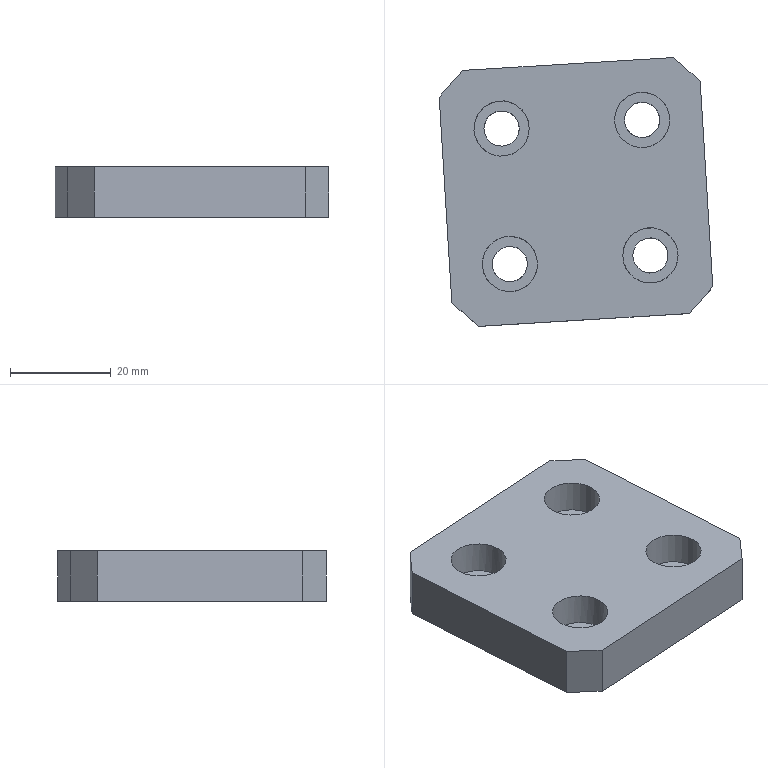Part | STEP file | 车灯-后视镜_id74_x_t | 1 solid | 22 faces | box 54.406 x 53.469 x 10 mm | volume 23010 mm3 | plane 14 | cylinder 8 | commonest cylinder face diameters 7 x4 11 x4
STEP:
#1=CARTESIAN_POINT('',(106.46,-55.923,-255.5));
#2=VERTEX_POINT('',#1);
#3=CARTESIAN_POINT('',(108.963,-96.847,-255.5));
#4=VERTEX_POINT('',#3);
#5=CARTESIAN_POINT('',(107.624,-74.965,-255.5));
#6=DIRECTION('',(0.06105,-0.9981,0.));
#7=VECTOR('',#6,1.);
#8=LINE('',#5,#7);
#9=EDGE_CURVE('',#2,#4,#8,.T.);
#10=ORIENTED_EDGE('',*,*,#9,.F.);
#11=CARTESIAN_POINT('',(101.164,-51.238,-255.5));
#12=VERTEX_POINT('',#11);
#13=CARTESIAN_POINT('',(94.843,-45.646,-255.5));
#14=DIRECTION('',(-0.749,0.6626,0.));
#15=VECTOR('',#14,1.);
#16=LINE('',#13,#15);
#17=EDGE_CURVE('',#2,#12,#16,.T.);
#18=ORIENTED_EDGE('',*,*,#17,.T.);
#19=CARTESIAN_POINT('',(59.242,-53.802,-255.5));
#20=VERTEX_POINT('',#19);
#21=CARTESIAN_POINT('',(65.219,-53.436,-255.5));
#22=DIRECTION('',(0.9981,0.06105,0.));
#23=VECTOR('',#22,1.);
#24=LINE('',#21,#23);
#25=EDGE_CURVE('',#20,#12,#24,.T.);
#26=ORIENTED_EDGE('',*,*,#25,.F.);
#27=CARTESIAN_POINT('',(54.557,-59.098,-255.5));
#28=VERTEX_POINT('',#27);
#29=CARTESIAN_POINT('',(50.767,-63.382,-255.5));
#30=DIRECTION('',(-0.6626,-0.749,0.));
#31=VECTOR('',#30,1.);
#32=LINE('',#29,#31);
#33=EDGE_CURVE('',#20,#28,#32,.T.);
#34=ORIENTED_EDGE('',*,*,#33,.T.);
#35=CARTESIAN_POINT('',(57.06,-100.021,-255.5));
#36=VERTEX_POINT('',#35);
#37=CARTESIAN_POINT('',(55.721,-78.139,-255.5));
#38=DIRECTION('',(-0.06105,0.9981,0.));
#39=VECTOR('',#38,1.);
#40=LINE('',#37,#39);
#41=EDGE_CURVE('',#36,#28,#40,.T.);
#42=ORIENTED_EDGE('',*,*,#41,.F.);
#43=CARTESIAN_POINT('',(62.355,-104.707,-255.5));
#44=VERTEX_POINT('',#43);
#45=CARTESIAN_POINT('',(51.269,-94.898,-255.5));
#46=DIRECTION('',(0.749,-0.6626,0.));
#47=VECTOR('',#46,1.);
#48=LINE('',#45,#47);
#49=EDGE_CURVE('',#36,#44,#48,.T.);
#50=ORIENTED_EDGE('',*,*,#49,.T.);
#51=CARTESIAN_POINT('',(104.277,-102.143,-255.5));
#52=VERTEX_POINT('',#51);
#53=CARTESIAN_POINT('',(68.333,-104.341,-255.5));
#54=DIRECTION('',(-0.9981,-0.06105,0.));
#55=VECTOR('',#54,1.);
#56=LINE('',#53,#55);
#57=EDGE_CURVE('',#52,#44,#56,.T.);
#58=ORIENTED_EDGE('',*,*,#57,.F.);
#59=CARTESIAN_POINT('',(100.019,-106.956,-255.5));
#60=DIRECTION('',(0.6626,0.749,0.));
#61=VECTOR('',#60,1.);
#62=LINE('',#59,#61);
#63=EDGE_CURVE('',#52,#4,#62,.T.);
#64=ORIENTED_EDGE('',*,*,#63,.T.);
#65=EDGE_LOOP('',(#10,#18,#26,#34,#42,#50,#58,#64));
#66=FACE_BOUND('',#65,.T.);
#67=CARTESIAN_POINT('',(74.11,-92.302,-255.5));
#68=VERTEX_POINT('',#67);
#69=CARTESIAN_POINT('',(68.61,-92.302,-255.5));
#70=DIRECTION('',(0.,0.,1.));
#71=DIRECTION('',(1.,0.,0.));
#72=AXIS2_PLACEMENT_3D('',#69,#70,#71);
#73=CIRCLE('',#72,5.5);
#74=EDGE_CURVE('',#68,#68,#73,.T.);
#75=ORIENTED_EDGE('',*,*,#74,.F.);
#76=EDGE_LOOP('',(#75));
#77=FACE_BOUND('',#76,.T.);
#78=CARTESIAN_POINT('',(102.058,-90.592,-255.5));
#79=VERTEX_POINT('',#78);
#80=CARTESIAN_POINT('',(96.558,-90.592,-255.5));
#81=DIRECTION('',(0.,0.,-1.));
#82=DIRECTION('',(1.,0.,0.));
#83=AXIS2_PLACEMENT_3D('',#80,#81,#82);
#84=CIRCLE('',#83,5.5);
#85=EDGE_CURVE('',#79,#79,#84,.T.);
#86=ORIENTED_EDGE('',*,*,#85,.T.);
#87=EDGE_LOOP('',(#86));
#88=FACE_BOUND('',#87,.T.);
#89=CARTESIAN_POINT('',(72.462,-65.352,-255.5));
#90=VERTEX_POINT('',#89);
#91=CARTESIAN_POINT('',(66.962,-65.352,-255.5));
#92=DIRECTION('',(0.,0.,-1.));
#93=DIRECTION('',(1.,0.,0.));
#94=AXIS2_PLACEMENT_3D('',#91,#92,#93);
#95=CIRCLE('',#94,5.5);
#96=EDGE_CURVE('',#90,#90,#95,.T.);
#97=ORIENTED_EDGE('',*,*,#96,.T.);
#98=EDGE_LOOP('',(#97));
#99=FACE_BOUND('',#98,.T.);
#100=CARTESIAN_POINT('',(100.409,-63.643,-255.5));
#101=VERTEX_POINT('',#100);
#102=CARTESIAN_POINT('',(94.909,-63.643,-255.5));
#103=DIRECTION('',(0.,0.,1.));
#104=DIRECTION('',(1.,0.,0.));
#105=AXIS2_PLACEMENT_3D('',#102,#103,#104);
#106=CIRCLE('',#105,5.5);
#107=EDGE_CURVE('',#101,#101,#106,.T.);
#108=ORIENTED_EDGE('',*,*,#107,.F.);
#109=EDGE_LOOP('',(#108));
#110=FACE_BOUND('',#109,.T.);
#111=CARTESIAN_POINT('',(66.689,-77.469,-255.5));
#112=DIRECTION('',(0.,0.,1.));
#113=DIRECTION('',(0.9981,0.06105,0.));
#114=AXIS2_PLACEMENT_3D('',#111,#112,#113);
#115=PLANE('',#114);
#116=ADVANCED_FACE('',(#66,#77,#88,#99,#110),#115,.T.);
#117=CARTESIAN_POINT('',(62.355,-104.707,-265.5));
#118=VERTEX_POINT('',#117);
#119=CARTESIAN_POINT('',(104.277,-102.143,-265.5));
#120=VERTEX_POINT('',#119);
#121=CARTESIAN_POINT('',(68.333,-104.341,-265.5));
#122=DIRECTION('',(0.9981,0.06105,0.));
#123=VECTOR('',#122,1.);
#124=LINE('',#121,#123);
#125=EDGE_CURVE('',#118,#120,#124,.T.);
#126=ORIENTED_EDGE('',*,*,#125,.T.);
#127=CARTESIAN_POINT('',(104.277,-102.143,-267.5));
#128=DIRECTION('',(0.,0.,1.));
#129=VECTOR('',#128,1.);
#130=LINE('',#127,#129);
#131=EDGE_CURVE('',#120,#52,#130,.T.);
#132=ORIENTED_EDGE('',*,*,#131,.T.);
#133=ORIENTED_EDGE('',*,*,#57,.T.);
#134=CARTESIAN_POINT('',(62.355,-104.707,-267.5));
#135=DIRECTION('',(0.,0.,-1.));
#136=VECTOR('',#135,1.);
#137=LINE('',#134,#136);
#138=EDGE_CURVE('',#44,#118,#137,.T.);
#139=ORIENTED_EDGE('',*,*,#138,.T.);
#140=EDGE_LOOP('',(#126,#132,#133,#139));
#141=FACE_OUTER_BOUND('',#140,.T.);
#142=CARTESIAN_POINT('',(68.333,-104.341,-267.5));
#143=DIRECTION('',(0.06105,-0.9981,0.));
#144=DIRECTION('',(0.,0.,-1.));
#145=AXIS2_PLACEMENT_3D('',#142,#143,#144);
#146=PLANE('',#145);
#147=ADVANCED_FACE('',(#141),#146,.T.);
#148=ORIENTED_EDGE('',*,*,#25,.T.);
#149=CARTESIAN_POINT('',(101.164,-51.238,-265.5));
#150=VERTEX_POINT('',#149);
#151=CARTESIAN_POINT('',(101.164,-51.238,-267.5));
#152=DIRECTION('',(0.,0.,-1.));
#153=VECTOR('',#152,1.);
#154=LINE('',#151,#153);
#155=EDGE_CURVE('',#12,#150,#154,.T.);
#156=ORIENTED_EDGE('',*,*,#155,.T.);
#157=CARTESIAN_POINT('',(59.242,-53.802,-265.5));
#158=VERTEX_POINT('',#157);
#159=CARTESIAN_POINT('',(65.219,-53.436,-265.5));
#160=DIRECTION('',(-0.9981,-0.06105,0.));
#161=VECTOR('',#160,1.);
#162=LINE('',#159,#161);
#163=EDGE_CURVE('',#150,#158,#162,.T.);
#164=ORIENTED_EDGE('',*,*,#163,.T.);
#165=CARTESIAN_POINT('',(59.242,-53.802,-267.5));
#166=DIRECTION('',(0.,0.,1.));
#167=VECTOR('',#166,1.);
#168=LINE('',#165,#167);
#169=EDGE_CURVE('',#158,#20,#168,.T.);
#170=ORIENTED_EDGE('',*,*,#169,.T.);
#171=EDGE_LOOP('',(#148,#156,#164,#170));
#172=FACE_OUTER_BOUND('',#171,.T.);
#173=CARTESIAN_POINT('',(65.219,-53.436,-267.5));
#174=DIRECTION('',(-0.06105,0.9981,0.));
#175=DIRECTION('',(0.,0.,1.));
#176=AXIS2_PLACEMENT_3D('',#173,#174,#175);
#177=PLANE('',#176);
#178=ADVANCED_FACE('',(#172),#177,.T.);
#179=ORIENTED_EDGE('',*,*,#163,.F.);
#180=CARTESIAN_POINT('',(106.46,-55.923,-265.5));
#181=VERTEX_POINT('',#180);
#182=CARTESIAN_POINT('',(94.843,-45.646,-265.5));
#183=DIRECTION('',(0.749,-0.6626,0.));
#184=VECTOR('',#183,1.);
#185=LINE('',#182,#184);
#186=EDGE_CURVE('',#150,#181,#185,.T.);
#187=ORIENTED_EDGE('',*,*,#186,.T.);
#188=CARTESIAN_POINT('',(108.963,-96.847,-265.5));
#189=VERTEX_POINT('',#188);
#190=CARTESIAN_POINT('',(107.624,-74.965,-265.5));
#191=DIRECTION('',(-0.06105,0.9981,0.));
#192=VECTOR('',#191,1.);
#193=LINE('',#190,#192);
#194=EDGE_CURVE('',#189,#181,#193,.T.);
#195=ORIENTED_EDGE('',*,*,#194,.F.);
#196=CARTESIAN_POINT('',(100.019,-106.956,-265.5));
#197=DIRECTION('',(-0.6626,-0.749,0.));
#198=VECTOR('',#197,1.);
#199=LINE('',#196,#198);
#200=EDGE_CURVE('',#189,#120,#199,.T.);
#201=ORIENTED_EDGE('',*,*,#200,.T.);
#202=ORIENTED_EDGE('',*,*,#125,.F.);
#203=CARTESIAN_POINT('',(57.06,-100.021,-265.5));
#204=VERTEX_POINT('',#203);
#205=CARTESIAN_POINT('',(51.269,-94.898,-265.5));
#206=DIRECTION('',(-0.749,0.6626,0.));
#207=VECTOR('',#206,1.);
#208=LINE('',#205,#207);
#209=EDGE_CURVE('',#118,#204,#208,.T.);
#210=ORIENTED_EDGE('',*,*,#209,.T.);
#211=CARTESIAN_POINT('',(54.557,-59.098,-265.5));
#212=VERTEX_POINT('',#211);
#213=CARTESIAN_POINT('',(55.721,-78.139,-265.5));
#214=DIRECTION('',(0.06105,-0.9981,0.));
#215=VECTOR('',#214,1.);
#216=LINE('',#213,#215);
#217=EDGE_CURVE('',#212,#204,#216,.T.);
#218=ORIENTED_EDGE('',*,*,#217,.F.);
#219=CARTESIAN_POINT('',(50.767,-63.382,-265.5));
#220=DIRECTION('',(0.6626,0.749,0.));
#221=VECTOR('',#220,1.);
#222=LINE('',#219,#221);
#223=EDGE_CURVE('',#212,#158,#222,.T.);
#224=ORIENTED_EDGE('',*,*,#223,.T.);
#225=EDGE_LOOP('',(#179,#187,#195,#201,#202,#210,#218,#224));
#226=FACE_BOUND('',#225,.T.);
#227=CARTESIAN_POINT('',(65.11,-92.302,-265.5));
#228=VERTEX_POINT('',#227);
#229=CARTESIAN_POINT('',(68.61,-92.302,-265.5));
#230=DIRECTION('',(0.,0.,-1.));
#231=DIRECTION('',(-1.,0.,0.));
#232=AXIS2_PLACEMENT_3D('',#229,#230,#231);
#233=CIRCLE('',#232,3.5);
#234=EDGE_CURVE('',#228,#228,#233,.T.);
#235=ORIENTED_EDGE('',*,*,#234,.F.);
#236=EDGE_LOOP('',(#235));
#237=FACE_BOUND('',#236,.T.);
#238=CARTESIAN_POINT('',(93.058,-90.592,-265.5));
#239=VERTEX_POINT('',#238);
#240=CARTESIAN_POINT('',(96.558,-90.592,-265.5));
#241=DIRECTION('',(0.,0.,1.));
#242=DIRECTION('',(-1.,0.,0.));
#243=AXIS2_PLACEMENT_3D('',#240,#241,#242);
#244=CIRCLE('',#243,3.5);
#245=EDGE_CURVE('',#239,#239,#244,.T.);
#246=ORIENTED_EDGE('',*,*,#245,.T.);
#247=EDGE_LOOP('',(#246));
#248=FACE_BOUND('',#247,.T.);
#249=CARTESIAN_POINT('',(63.462,-65.352,-265.5));
#250=VERTEX_POINT('',#249);
#251=CARTESIAN_POINT('',(66.962,-65.352,-265.5));
#252=DIRECTION('',(0.,0.,1.));
#253=DIRECTION('',(-1.,0.,0.));
#254=AXIS2_PLACEMENT_3D('',#251,#252,#253);
#255=CIRCLE('',#254,3.5);
#256=EDGE_CURVE('',#250,#250,#255,.T.);
#257=ORIENTED_EDGE('',*,*,#256,.T.);
#258=EDGE_LOOP('',(#257));
#259=FACE_BOUND('',#258,.T.);
#260=CARTESIAN_POINT('',(91.409,-63.643,-265.5));
#261=VERTEX_POINT('',#260);
#262=CARTESIAN_POINT('',(94.909,-63.643,-265.5));
#263=DIRECTION('',(0.,0.,-1.));
#264=DIRECTION('',(-1.,0.,0.));
#265=AXIS2_PLACEMENT_3D('',#262,#263,#264);
#266=CIRCLE('',#265,3.5);
#267=EDGE_CURVE('',#261,#261,#266,.T.);
#268=ORIENTED_EDGE('',*,*,#267,.F.);
#269=EDGE_LOOP('',(#268));
#270=FACE_BOUND('',#269,.T.);
#271=CARTESIAN_POINT('',(66.689,-77.469,-265.5));
#272=DIRECTION('',(0.,0.,-1.));
#273=DIRECTION('',(-0.9981,-0.06105,0.));
#274=AXIS2_PLACEMENT_3D('',#271,#272,#273);
#275=PLANE('',#274);
#276=ADVANCED_FACE('',(#226,#237,#248,#259,#270),#275,.T.);
#277=ORIENTED_EDGE('',*,*,#194,.T.);
#278=CARTESIAN_POINT('',(106.46,-55.923,-267.5));
#279=DIRECTION('',(0.,0.,1.));
#280=VECTOR('',#279,1.);
#281=LINE('',#278,#280);
#282=EDGE_CURVE('',#181,#2,#281,.T.);
#283=ORIENTED_EDGE('',*,*,#282,.T.);
#284=ORIENTED_EDGE('',*,*,#9,.T.);
#285=CARTESIAN_POINT('',(108.963,-96.847,-267.5));
#286=DIRECTION('',(0.,0.,-1.));
#287=VECTOR('',#286,1.);
#288=LINE('',#285,#287);
#289=EDGE_CURVE('',#4,#189,#288,.T.);
#290=ORIENTED_EDGE('',*,*,#289,.T.);
#291=EDGE_LOOP('',(#277,#283,#284,#290));
#292=FACE_OUTER_BOUND('',#291,.T.);
#293=CARTESIAN_POINT('',(107.624,-74.965,-267.5));
#294=DIRECTION('',(0.9981,0.06105,0.));
#295=DIRECTION('',(0.,0.,-1.));
#296=AXIS2_PLACEMENT_3D('',#293,#294,#295);
#297=PLANE('',#296);
#298=ADVANCED_FACE('',(#292),#297,.T.);
#299=CARTESIAN_POINT('',(91.416,-63.857,-262.));
#300=VERTEX_POINT('',#299);
#301=CARTESIAN_POINT('',(94.909,-63.643,-262.));
#302=DIRECTION('',(0.,0.,-1.));
#303=DIRECTION('',(-0.9981,-0.06105,0.));
#304=AXIS2_PLACEMENT_3D('',#301,#302,#303);
#305=CIRCLE('',#304,3.5);
#306=EDGE_CURVE('',#300,#300,#305,.T.);
#307=ORIENTED_EDGE('',*,*,#306,.F.);
#308=EDGE_LOOP('',(#307));
#309=FACE_BOUND('',#308,.T.);
#310=ORIENTED_EDGE('',*,*,#267,.T.);
#311=EDGE_LOOP('',(#310));
#312=FACE_BOUND('',#311,.T.);
#313=CARTESIAN_POINT('',(94.909,-63.643,-265.5));
#314=DIRECTION('',(0.,0.,1.));
#315=DIRECTION('',(-0.9981,-0.06105,0.));
#316=AXIS2_PLACEMENT_3D('',#313,#314,#315);
#317=CYLINDRICAL_SURFACE('',#316,3.5);
#318=ADVANCED_FACE('',(#309,#312),#317,.F.);
#319=ORIENTED_EDGE('',*,*,#306,.T.);
#320=EDGE_LOOP('',(#319));
#321=FACE_BOUND('',#320,.T.);
#322=CARTESIAN_POINT('',(89.42,-63.979,-262.));
#323=VERTEX_POINT('',#322);
#324=CARTESIAN_POINT('',(94.909,-63.643,-262.));
#325=DIRECTION('',(0.,0.,-1.));
#326=DIRECTION('',(-0.9981,-0.06105,0.));
#327=AXIS2_PLACEMENT_3D('',#324,#325,#326);
#328=CIRCLE('',#327,5.5);
#329=EDGE_CURVE('',#323,#323,#328,.T.);
#330=ORIENTED_EDGE('',*,*,#329,.F.);
#331=EDGE_LOOP('',(#330));
#332=FACE_BOUND('',#331,.T.);
#333=CARTESIAN_POINT('',(94.909,-63.643,-262.));
#334=DIRECTION('',(0.,0.,-1.));
#335=DIRECTION('',(0.9981,0.06105,0.));
#336=AXIS2_PLACEMENT_3D('',#333,#334,#335);
#337=PLANE('',#336);
#338=ADVANCED_FACE('',(#321,#332),#337,.F.);
#339=ORIENTED_EDGE('',*,*,#329,.T.);
#340=EDGE_LOOP('',(#339));
#341=FACE_BOUND('',#340,.T.);
#342=ORIENTED_EDGE('',*,*,#107,.T.);
#343=EDGE_LOOP('',(#342));
#344=FACE_BOUND('',#343,.T.);
#345=CARTESIAN_POINT('',(94.909,-63.643,-255.5));
#346=DIRECTION('',(0.,0.,-1.));
#347=DIRECTION('',(0.9981,0.06105,0.));
#348=AXIS2_PLACEMENT_3D('',#345,#346,#347);
#349=CYLINDRICAL_SURFACE('',#348,5.5);
#350=ADVANCED_FACE('',(#341,#344),#349,.F.);
#351=CARTESIAN_POINT('',(63.468,-65.566,-262.));
#352=VERTEX_POINT('',#351);
#353=CARTESIAN_POINT('',(66.962,-65.352,-262.));
#354=DIRECTION('',(0.,0.,1.));
#355=DIRECTION('',(-0.9981,-0.06105,0.));
#356=AXIS2_PLACEMENT_3D('',#353,#354,#355);
#357=CIRCLE('',#356,3.5);
#358=EDGE_CURVE('',#352,#352,#357,.T.);
#359=ORIENTED_EDGE('',*,*,#358,.T.);
#360=EDGE_LOOP('',(#359));
#361=FACE_BOUND('',#360,.T.);
#362=ORIENTED_EDGE('',*,*,#256,.F.);
#363=EDGE_LOOP('',(#362));
#364=FACE_BOUND('',#363,.T.);
#365=CARTESIAN_POINT('',(66.962,-65.352,-265.5));
#366=DIRECTION('',(0.,0.,1.));
#367=DIRECTION('',(0.9981,0.06105,0.));
#368=AXIS2_PLACEMENT_3D('',#365,#366,#367);
#369=CYLINDRICAL_SURFACE('',#368,3.5);
#370=ADVANCED_FACE('',(#361,#364),#369,.F.);
#371=ORIENTED_EDGE('',*,*,#358,.F.);
#372=EDGE_LOOP('',(#371));
#373=FACE_BOUND('',#372,.T.);
#374=CARTESIAN_POINT('',(61.472,-65.688,-262.));
#375=VERTEX_POINT('',#374);
#376=CARTESIAN_POINT('',(66.962,-65.352,-262.));
#377=DIRECTION('',(0.,0.,1.));
#378=DIRECTION('',(-0.9981,-0.06105,0.));
#379=AXIS2_PLACEMENT_3D('',#376,#377,#378);
#380=CIRCLE('',#379,5.5);
#381=EDGE_CURVE('',#375,#375,#380,.T.);
#382=ORIENTED_EDGE('',*,*,#381,.T.);
#383=EDGE_LOOP('',(#382));
#384=FACE_BOUND('',#383,.T.);
#385=CARTESIAN_POINT('',(66.962,-65.352,-262.));
#386=DIRECTION('',(0.,0.,-1.));
#387=DIRECTION('',(-0.9981,-0.06105,0.));
#388=AXIS2_PLACEMENT_3D('',#385,#386,#387);
#389=PLANE('',#388);
#390=ADVANCED_FACE('',(#373,#384),#389,.F.);
#391=ORIENTED_EDGE('',*,*,#381,.F.);
#392=EDGE_LOOP('',(#391));
#393=FACE_BOUND('',#392,.T.);
#394=ORIENTED_EDGE('',*,*,#96,.F.);
#395=EDGE_LOOP('',(#394));
#396=FACE_BOUND('',#395,.T.);
#397=CARTESIAN_POINT('',(66.962,-65.352,-255.5));
#398=DIRECTION('',(0.,0.,-1.));
#399=DIRECTION('',(-0.9981,-0.06105,0.));
#400=AXIS2_PLACEMENT_3D('',#397,#398,#399);
#401=CYLINDRICAL_SURFACE('',#400,5.5);
#402=ADVANCED_FACE('',(#393,#396),#401,.F.);
#403=CARTESIAN_POINT('',(93.064,-90.806,-262.));
#404=VERTEX_POINT('',#403);
#405=CARTESIAN_POINT('',(96.558,-90.592,-262.));
#406=DIRECTION('',(0.,0.,1.));
#407=DIRECTION('',(-0.9981,-0.06105,0.));
#408=AXIS2_PLACEMENT_3D('',#405,#406,#407);
#409=CIRCLE('',#408,3.5);
#410=EDGE_CURVE('',#404,#404,#409,.T.);
#411=ORIENTED_EDGE('',*,*,#410,.T.);
#412=EDGE_LOOP('',(#411));
#413=FACE_BOUND('',#412,.T.);
#414=ORIENTED_EDGE('',*,*,#245,.F.);
#415=EDGE_LOOP('',(#414));
#416=FACE_BOUND('',#415,.T.);
#417=CARTESIAN_POINT('',(96.558,-90.592,-265.5));
#418=DIRECTION('',(0.,0.,1.));
#419=DIRECTION('',(-0.9981,-0.06105,0.));
#420=AXIS2_PLACEMENT_3D('',#417,#418,#419);
#421=CYLINDRICAL_SURFACE('',#420,3.5);
#422=ADVANCED_FACE('',(#413,#416),#421,.F.);
#423=ORIENTED_EDGE('',*,*,#410,.F.);
#424=EDGE_LOOP('',(#423));
#425=FACE_BOUND('',#424,.T.);
#426=CARTESIAN_POINT('',(91.068,-90.928,-262.));
#427=VERTEX_POINT('',#426);
#428=CARTESIAN_POINT('',(96.558,-90.592,-262.));
#429=DIRECTION('',(0.,0.,1.));
#430=DIRECTION('',(-0.9981,-0.06105,0.));
#431=AXIS2_PLACEMENT_3D('',#428,#429,#430);
#432=CIRCLE('',#431,5.5);
#433=EDGE_CURVE('',#427,#427,#432,.T.);
#434=ORIENTED_EDGE('',*,*,#433,.T.);
#435=EDGE_LOOP('',(#434));
#436=FACE_BOUND('',#435,.T.);
#437=CARTESIAN_POINT('',(96.558,-90.592,-262.));
#438=DIRECTION('',(0.,0.,-1.));
#439=DIRECTION('',(0.9981,0.06105,0.));
#440=AXIS2_PLACEMENT_3D('',#437,#438,#439);
#441=PLANE('',#440);
#442=ADVANCED_FACE('',(#425,#436),#441,.F.);
#443=ORIENTED_EDGE('',*,*,#433,.F.);
#444=EDGE_LOOP('',(#443));
#445=FACE_BOUND('',#444,.T.);
#446=ORIENTED_EDGE('',*,*,#85,.F.);
#447=EDGE_LOOP('',(#446));
#448=FACE_BOUND('',#447,.T.);
#449=CARTESIAN_POINT('',(96.558,-90.592,-255.5));
#450=DIRECTION('',(0.,0.,-1.));
#451=DIRECTION('',(0.9981,0.06105,0.));
#452=AXIS2_PLACEMENT_3D('',#449,#450,#451);
#453=CYLINDRICAL_SURFACE('',#452,5.5);
#454=ADVANCED_FACE('',(#445,#448),#453,.F.);
#455=CARTESIAN_POINT('',(65.116,-92.516,-262.));
#456=VERTEX_POINT('',#455);
#457=CARTESIAN_POINT('',(68.61,-92.302,-262.));
#458=DIRECTION('',(0.,0.,-1.));
#459=DIRECTION('',(-0.9981,-0.06105,0.));
#460=AXIS2_PLACEMENT_3D('',#457,#458,#459);
#461=CIRCLE('',#460,3.5);
#462=EDGE_CURVE('',#456,#456,#461,.T.);
#463=ORIENTED_EDGE('',*,*,#462,.F.);
#464=EDGE_LOOP('',(#463));
#465=FACE_BOUND('',#464,.T.);
#466=ORIENTED_EDGE('',*,*,#234,.T.);
#467=EDGE_LOOP('',(#466));
#468=FACE_BOUND('',#467,.T.);
#469=CARTESIAN_POINT('',(68.61,-92.302,-265.5));
#470=DIRECTION('',(0.,0.,1.));
#471=DIRECTION('',(0.9981,0.06105,0.));
#472=AXIS2_PLACEMENT_3D('',#469,#470,#471);
#473=CYLINDRICAL_SURFACE('',#472,3.5);
#474=ADVANCED_FACE('',(#465,#468),#473,.F.);
#475=ORIENTED_EDGE('',*,*,#462,.T.);
#476=EDGE_LOOP('',(#475));
#477=FACE_BOUND('',#476,.T.);
#478=CARTESIAN_POINT('',(63.12,-92.638,-262.));
#479=VERTEX_POINT('',#478);
#480=CARTESIAN_POINT('',(68.61,-92.302,-262.));
#481=DIRECTION('',(0.,0.,-1.));
#482=DIRECTION('',(-0.9981,-0.06105,0.));
#483=AXIS2_PLACEMENT_3D('',#480,#481,#482);
#484=CIRCLE('',#483,5.5);
#485=EDGE_CURVE('',#479,#479,#484,.T.);
#486=ORIENTED_EDGE('',*,*,#485,.F.);
#487=EDGE_LOOP('',(#486));
#488=FACE_BOUND('',#487,.T.);
#489=CARTESIAN_POINT('',(68.61,-92.302,-262.));
#490=DIRECTION('',(0.,0.,-1.));
#491=DIRECTION('',(-0.9981,-0.06105,0.));
#492=AXIS2_PLACEMENT_3D('',#489,#490,#491);
#493=PLANE('',#492);
#494=ADVANCED_FACE('',(#477,#488),#493,.F.);
#495=ORIENTED_EDGE('',*,*,#485,.T.);
#496=EDGE_LOOP('',(#495));
#497=FACE_BOUND('',#496,.T.);
#498=ORIENTED_EDGE('',*,*,#74,.T.);
#499=EDGE_LOOP('',(#498));
#500=FACE_BOUND('',#499,.T.);
#501=CARTESIAN_POINT('',(68.61,-92.302,-255.5));
#502=DIRECTION('',(0.,0.,-1.));
#503=DIRECTION('',(-0.9981,-0.06105,0.));
#504=AXIS2_PLACEMENT_3D('',#501,#502,#503);
#505=CYLINDRICAL_SURFACE('',#504,5.5);
#506=ADVANCED_FACE('',(#497,#500),#505,.F.);
#507=ORIENTED_EDGE('',*,*,#217,.T.);
#508=CARTESIAN_POINT('',(57.06,-100.021,-261.5));
#509=DIRECTION('',(0.,0.,1.));
#510=VECTOR('',#509,1.);
#511=LINE('',#508,#510);
#512=EDGE_CURVE('',#204,#36,#511,.T.);
#513=ORIENTED_EDGE('',*,*,#512,.T.);
#514=ORIENTED_EDGE('',*,*,#41,.T.);
#515=CARTESIAN_POINT('',(54.557,-59.098,-261.5));
#516=DIRECTION('',(0.,0.,-1.));
#517=VECTOR('',#516,1.);
#518=LINE('',#515,#517);
#519=EDGE_CURVE('',#28,#212,#518,.T.);
#520=ORIENTED_EDGE('',*,*,#519,.T.);
#521=EDGE_LOOP('',(#507,#513,#514,#520));
#522=FACE_OUTER_BOUND('',#521,.T.);
#523=CARTESIAN_POINT('',(55.721,-78.139,-261.5));
#524=DIRECTION('',(0.9981,0.06105,0.));
#525=DIRECTION('',(0.,0.,1.));
#526=AXIS2_PLACEMENT_3D('',#523,#524,#525);
#527=PLANE('',#526);
#528=ADVANCED_FACE('',(#522),#527,.F.);
#529=ORIENTED_EDGE('',*,*,#209,.F.);
#530=ORIENTED_EDGE('',*,*,#138,.F.);
#531=ORIENTED_EDGE('',*,*,#49,.F.);
#532=ORIENTED_EDGE('',*,*,#512,.F.);
#533=EDGE_LOOP('',(#529,#530,#531,#532));
#534=FACE_OUTER_BOUND('',#533,.T.);
#535=CARTESIAN_POINT('',(57.06,-100.021,-261.5));
#536=DIRECTION('',(-0.6626,-0.749,0.));
#537=DIRECTION('',(0.749,-0.6626,0.));
#538=AXIS2_PLACEMENT_3D('',#535,#536,#537);
#539=PLANE('',#538);
#540=ADVANCED_FACE('',(#534),#539,.T.);
#541=ORIENTED_EDGE('',*,*,#33,.F.);
#542=ORIENTED_EDGE('',*,*,#169,.F.);
#543=ORIENTED_EDGE('',*,*,#223,.F.);
#544=ORIENTED_EDGE('',*,*,#519,.F.);
#545=EDGE_LOOP('',(#541,#542,#543,#544));
#546=FACE_OUTER_BOUND('',#545,.T.);
#547=CARTESIAN_POINT('',(54.557,-59.098,-261.5));
#548=DIRECTION('',(-0.749,0.6626,0.));
#549=DIRECTION('',(-0.6626,-0.749,0.));
#550=AXIS2_PLACEMENT_3D('',#547,#548,#549);
#551=PLANE('',#550);
#552=ADVANCED_FACE('',(#546),#551,.T.);
#553=ORIENTED_EDGE('',*,*,#17,.F.);
#554=ORIENTED_EDGE('',*,*,#282,.F.);
#555=ORIENTED_EDGE('',*,*,#186,.F.);
#556=ORIENTED_EDGE('',*,*,#155,.F.);
#557=EDGE_LOOP('',(#553,#554,#555,#556));
#558=FACE_OUTER_BOUND('',#557,.T.);
#559=CARTESIAN_POINT('',(101.164,-51.238,-267.5));
#560=DIRECTION('',(-0.6626,-0.749,0.));
#561=DIRECTION('',(0.749,-0.6626,0.));
#562=AXIS2_PLACEMENT_3D('',#559,#560,#561);
#563=PLANE('',#562);
#564=ADVANCED_FACE('',(#558),#563,.F.);
#565=ORIENTED_EDGE('',*,*,#63,.F.);
#566=ORIENTED_EDGE('',*,*,#131,.F.);
#567=ORIENTED_EDGE('',*,*,#200,.F.);
#568=ORIENTED_EDGE('',*,*,#289,.F.);
#569=EDGE_LOOP('',(#565,#566,#567,#568));
#570=FACE_OUTER_BOUND('',#569,.T.);
#571=CARTESIAN_POINT('',(108.963,-96.847,-267.5));
#572=DIRECTION('',(-0.749,0.6626,0.));
#573=DIRECTION('',(-0.6626,-0.749,0.));
#574=AXIS2_PLACEMENT_3D('',#571,#572,#573);
#575=PLANE('',#574);
#576=ADVANCED_FACE('',(#570),#575,.F.);
#577=CLOSED_SHELL('',(#116,#147,#178,#276,#298,#318,#338,#350,#370,#390,#402,#422,#442,#454,#474,#494,#506,#528,#540,#552,#564,#576));
#578=MANIFOLD_SOLID_BREP('',#577);
#579=(LENGTH_UNIT()NAMED_UNIT(*)SI_UNIT(.MILLI.,.METRE.));
#580=UNCERTAINTY_MEASURE_WITH_UNIT(LENGTH_MEASURE(0.00002),#579,'','');
#581=(NAMED_UNIT(*)PLANE_ANGLE_UNIT()SI_UNIT($,.RADIAN.));
#582=PLANE_ANGLE_MEASURE_WITH_UNIT(PLANE_ANGLE_MEASURE(0.01745),#581);
#583=DIMENSIONAL_EXPONENTS(0.,0.,0.,0.,0.,0.,0.);
#584=(CONVERSION_BASED_UNIT('DEGREE',#582)NAMED_UNIT(#583)PLANE_ANGLE_UNIT());
#585=(NAMED_UNIT(*)SI_UNIT($,.STERADIAN.)SOLID_ANGLE_UNIT());
#586=(GEOMETRIC_REPRESENTATION_CONTEXT(3)GLOBAL_UNCERTAINTY_ASSIGNED_CONTEXT((#580))GLOBAL_UNIT_ASSIGNED_CONTEXT((#579,#584,#585))REPRESENTATION_CONTEXT('',''));
#587=ADVANCED_BREP_SHAPE_REPRESENTATION('',(#578),#586);